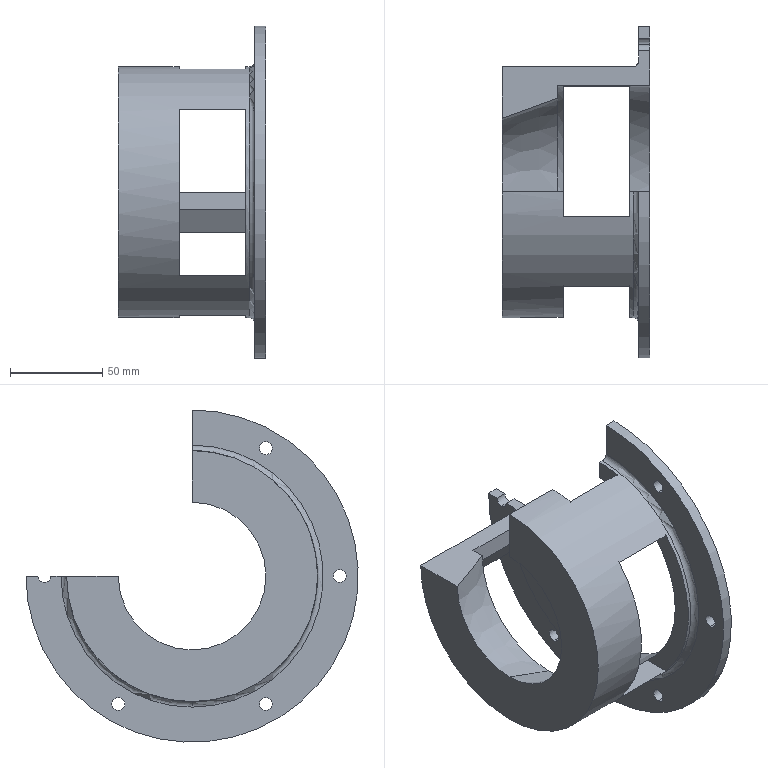Part | SolidWorks | features ICE 3, CirPattern 1, Fillet 1, Revolution 1 | 1 solid | 36 faces | box 80 x 180 x 180 mm | volume 298763 mm3 | plane 19 | cylinder 13 | torus 2 | cone 2 | commonest cylinder face diameters 7 x10 116 x1 136 x1 180 x1
STEP:
#1=CARTESIAN_POINT('',(74.,0.,-71.));
#2=VERTEX_POINT('',#1);
#3=CARTESIAN_POINT('',(74.,71.,0.));
#4=VERTEX_POINT('',#3);
#5=CARTESIAN_POINT('',(74.,0.,0.));
#6=DIRECTION('',(1.,0.,0.));
#7=DIRECTION('',(0.,0.,-1.));
#8=AXIS2_PLACEMENT_3D('',#5,#6,#7);
#9=CIRCLE('',#8,71.);
#10=EDGE_CURVE('',#2,#4,#9,.T.);
#11=ORIENTED_EDGE('',*,*,#10,.F.);
#12=CARTESIAN_POINT('',(71.,0.,-68.));
#13=VERTEX_POINT('',#12);
#14=CARTESIAN_POINT('',(71.,0.,-71.));
#15=DIRECTION('',(0.,-1.,0.));
#16=DIRECTION('',(0.,0.,-1.));
#17=AXIS2_PLACEMENT_3D('',#14,#15,#16);
#18=CIRCLE('',#17,3.);
#19=EDGE_CURVE('',#2,#13,#18,.T.);
#20=ORIENTED_EDGE('',*,*,#19,.T.);
#21=CARTESIAN_POINT('',(71.,68.,0.));
#22=VERTEX_POINT('',#21);
#23=CARTESIAN_POINT('',(71.,0.,0.));
#24=DIRECTION('',(-1.,0.,0.));
#25=DIRECTION('',(0.,0.,-1.));
#26=AXIS2_PLACEMENT_3D('',#23,#24,#25);
#27=CIRCLE('',#26,68.);
#28=EDGE_CURVE('',#22,#13,#27,.T.);
#29=ORIENTED_EDGE('',*,*,#28,.F.);
#30=CARTESIAN_POINT('',(71.,71.,0.));
#31=DIRECTION('',(0.,0.,1.));
#32=DIRECTION('',(-1.,0.,0.));
#33=AXIS2_PLACEMENT_3D('',#30,#31,#32);
#34=CIRCLE('',#33,3.);
#35=EDGE_CURVE('',#22,#4,#34,.T.);
#36=ORIENTED_EDGE('',*,*,#35,.T.);
#37=EDGE_LOOP('',(#11,#20,#29,#36));
#38=FACE_OUTER_BOUND('',#37,.T.);
#39=CARTESIAN_POINT('',(71.,0.,0.));
#40=DIRECTION('',(1.,0.,0.));
#41=DIRECTION('',(0.,0.,-1.));
#42=AXIS2_PLACEMENT_3D('',#39,#40,#41);
#43=TOROIDAL_SURFACE('',#42,71.,3.);
#44=ADVANCED_FACE('',(#38),#43,.F.);
#45=CARTESIAN_POINT('',(74.,40.,-65.782));
#46=VERTEX_POINT('',#45);
#47=CARTESIAN_POINT('',(74.,40.,-72.782));
#48=VERTEX_POINT('',#47);
#49=CARTESIAN_POINT('',(74.,40.,-69.282));
#50=DIRECTION('',(1.,0.,0.));
#51=DIRECTION('',(0.,0.,-1.));
#52=AXIS2_PLACEMENT_3D('',#49,#50,#51);
#53=CIRCLE('',#52,3.5);
#54=EDGE_CURVE('',#46,#48,#53,.T.);
#55=ORIENTED_EDGE('',*,*,#54,.F.);
#56=CARTESIAN_POINT('',(80.,40.,-65.782));
#57=VERTEX_POINT('',#56);
#58=CARTESIAN_POINT('',(70.,40.,-65.782));
#59=DIRECTION('',(1.,0.,0.));
#60=VECTOR('',#59,1000.);
#61=LINE('',#58,#60);
#62=EDGE_CURVE('',#46,#57,#61,.T.);
#63=ORIENTED_EDGE('',*,*,#62,.T.);
#64=CARTESIAN_POINT('',(80.,40.,-72.782));
#65=VERTEX_POINT('',#64);
#66=CARTESIAN_POINT('',(80.,40.,-69.282));
#67=DIRECTION('',(1.,0.,0.));
#68=DIRECTION('',(0.,0.,-1.));
#69=AXIS2_PLACEMENT_3D('',#66,#67,#68);
#70=CIRCLE('',#69,3.5);
#71=EDGE_CURVE('',#57,#65,#70,.T.);
#72=ORIENTED_EDGE('',*,*,#71,.T.);
#73=CARTESIAN_POINT('',(70.,40.,-72.782));
#74=DIRECTION('',(1.,0.,0.));
#75=VECTOR('',#74,1000.);
#76=LINE('',#73,#75);
#77=EDGE_CURVE('',#48,#65,#76,.T.);
#78=ORIENTED_EDGE('',*,*,#77,.F.);
#79=EDGE_LOOP('',(#55,#63,#72,#78));
#80=FACE_OUTER_BOUND('',#79,.T.);
#81=CARTESIAN_POINT('',(70.,40.,-69.282));
#82=DIRECTION('',(1.,0.,0.));
#83=DIRECTION('',(0.,0.,-1.));
#84=AXIS2_PLACEMENT_3D('',#81,#82,#83);
#85=CYLINDRICAL_SURFACE('',#84,3.5);
#86=ADVANCED_FACE('',(#80),#85,.F.);
#87=CARTESIAN_POINT('',(74.,-40.,-65.782));
#88=VERTEX_POINT('',#87);
#89=CARTESIAN_POINT('',(74.,-40.,-72.782));
#90=VERTEX_POINT('',#89);
#91=CARTESIAN_POINT('',(74.,-40.,-69.282));
#92=DIRECTION('',(1.,0.,0.));
#93=DIRECTION('',(0.,0.,-1.));
#94=AXIS2_PLACEMENT_3D('',#91,#92,#93);
#95=CIRCLE('',#94,3.5);
#96=EDGE_CURVE('',#88,#90,#95,.T.);
#97=ORIENTED_EDGE('',*,*,#96,.F.);
#98=CARTESIAN_POINT('',(80.,-40.,-65.782));
#99=VERTEX_POINT('',#98);
#100=CARTESIAN_POINT('',(70.,-40.,-65.782));
#101=DIRECTION('',(1.,0.,0.));
#102=VECTOR('',#101,1000.);
#103=LINE('',#100,#102);
#104=EDGE_CURVE('',#88,#99,#103,.T.);
#105=ORIENTED_EDGE('',*,*,#104,.T.);
#106=CARTESIAN_POINT('',(80.,-40.,-72.782));
#107=VERTEX_POINT('',#106);
#108=CARTESIAN_POINT('',(80.,-40.,-69.282));
#109=DIRECTION('',(1.,0.,0.));
#110=DIRECTION('',(0.,0.,-1.));
#111=AXIS2_PLACEMENT_3D('',#108,#109,#110);
#112=CIRCLE('',#111,3.5);
#113=EDGE_CURVE('',#99,#107,#112,.T.);
#114=ORIENTED_EDGE('',*,*,#113,.T.);
#115=CARTESIAN_POINT('',(70.,-40.,-72.782));
#116=DIRECTION('',(1.,0.,0.));
#117=VECTOR('',#116,1000.);
#118=LINE('',#115,#117);
#119=EDGE_CURVE('',#90,#107,#118,.T.);
#120=ORIENTED_EDGE('',*,*,#119,.F.);
#121=EDGE_LOOP('',(#97,#105,#114,#120));
#122=FACE_OUTER_BOUND('',#121,.T.);
#123=CARTESIAN_POINT('',(70.,-40.,-69.282));
#124=DIRECTION('',(1.,0.,0.));
#125=DIRECTION('',(0.,0.,-1.));
#126=AXIS2_PLACEMENT_3D('',#123,#124,#125);
#127=CYLINDRICAL_SURFACE('',#126,3.5);
#128=ADVANCED_FACE('',(#122),#127,.F.);
#129=CARTESIAN_POINT('',(74.,-80.,3.5));
#130=VERTEX_POINT('',#129);
#131=CARTESIAN_POINT('',(74.,-80.,-3.5));
#132=VERTEX_POINT('',#131);
#133=CARTESIAN_POINT('',(74.,-80.,0.));
#134=DIRECTION('',(1.,0.,0.));
#135=DIRECTION('',(0.,0.,-1.));
#136=AXIS2_PLACEMENT_3D('',#133,#134,#135);
#137=CIRCLE('',#136,3.5);
#138=EDGE_CURVE('',#130,#132,#137,.T.);
#139=ORIENTED_EDGE('',*,*,#138,.F.);
#140=CARTESIAN_POINT('',(80.,-80.,3.5));
#141=VERTEX_POINT('',#140);
#142=CARTESIAN_POINT('',(70.,-80.,3.5));
#143=DIRECTION('',(1.,0.,0.));
#144=VECTOR('',#143,1000.);
#145=LINE('',#142,#144);
#146=EDGE_CURVE('',#130,#141,#145,.T.);
#147=ORIENTED_EDGE('',*,*,#146,.T.);
#148=CARTESIAN_POINT('',(80.,-80.,-3.5));
#149=VERTEX_POINT('',#148);
#150=CARTESIAN_POINT('',(80.,-80.,0.));
#151=DIRECTION('',(1.,0.,0.));
#152=DIRECTION('',(0.,0.,-1.));
#153=AXIS2_PLACEMENT_3D('',#150,#151,#152);
#154=CIRCLE('',#153,3.5);
#155=EDGE_CURVE('',#141,#149,#154,.T.);
#156=ORIENTED_EDGE('',*,*,#155,.T.);
#157=CARTESIAN_POINT('',(70.,-80.,-3.5));
#158=DIRECTION('',(1.,0.,0.));
#159=VECTOR('',#158,1000.);
#160=LINE('',#157,#159);
#161=EDGE_CURVE('',#132,#149,#160,.T.);
#162=ORIENTED_EDGE('',*,*,#161,.F.);
#163=EDGE_LOOP('',(#139,#147,#156,#162));
#164=FACE_OUTER_BOUND('',#163,.T.);
#165=CARTESIAN_POINT('',(70.,-80.,0.));
#166=DIRECTION('',(1.,0.,0.));
#167=DIRECTION('',(0.,0.,-1.));
#168=AXIS2_PLACEMENT_3D('',#165,#166,#167);
#169=CYLINDRICAL_SURFACE('',#168,3.5);
#170=ADVANCED_FACE('',(#164),#169,.F.);
#171=CARTESIAN_POINT('',(74.,-40.,72.782));
#172=VERTEX_POINT('',#171);
#173=CARTESIAN_POINT('',(74.,-40.,65.782));
#174=VERTEX_POINT('',#173);
#175=CARTESIAN_POINT('',(74.,-40.,69.282));
#176=DIRECTION('',(1.,0.,0.));
#177=DIRECTION('',(0.,0.,-1.));
#178=AXIS2_PLACEMENT_3D('',#175,#176,#177);
#179=CIRCLE('',#178,3.5);
#180=EDGE_CURVE('',#172,#174,#179,.T.);
#181=ORIENTED_EDGE('',*,*,#180,.F.);
#182=CARTESIAN_POINT('',(80.,-40.,72.782));
#183=VERTEX_POINT('',#182);
#184=CARTESIAN_POINT('',(70.,-40.,72.782));
#185=DIRECTION('',(1.,0.,0.));
#186=VECTOR('',#185,1000.);
#187=LINE('',#184,#186);
#188=EDGE_CURVE('',#172,#183,#187,.T.);
#189=ORIENTED_EDGE('',*,*,#188,.T.);
#190=CARTESIAN_POINT('',(80.,-40.,65.782));
#191=VERTEX_POINT('',#190);
#192=CARTESIAN_POINT('',(80.,-40.,69.282));
#193=DIRECTION('',(1.,0.,0.));
#194=DIRECTION('',(0.,0.,-1.));
#195=AXIS2_PLACEMENT_3D('',#192,#193,#194);
#196=CIRCLE('',#195,3.5);
#197=EDGE_CURVE('',#183,#191,#196,.T.);
#198=ORIENTED_EDGE('',*,*,#197,.T.);
#199=CARTESIAN_POINT('',(70.,-40.,65.782));
#200=DIRECTION('',(1.,0.,0.));
#201=VECTOR('',#200,1000.);
#202=LINE('',#199,#201);
#203=EDGE_CURVE('',#174,#191,#202,.T.);
#204=ORIENTED_EDGE('',*,*,#203,.F.);
#205=EDGE_LOOP('',(#181,#189,#198,#204));
#206=FACE_OUTER_BOUND('',#205,.T.);
#207=CARTESIAN_POINT('',(70.,-40.,69.282));
#208=DIRECTION('',(1.,0.,0.));
#209=DIRECTION('',(0.,0.,-1.));
#210=AXIS2_PLACEMENT_3D('',#207,#208,#209);
#211=CYLINDRICAL_SURFACE('',#210,3.5);
#212=ADVANCED_FACE('',(#206),#211,.F.);
#213=CARTESIAN_POINT('',(74.,80.,-3.5));
#214=VERTEX_POINT('',#213);
#215=CARTESIAN_POINT('',(74.,83.5,0.));
#216=VERTEX_POINT('',#215);
#217=CARTESIAN_POINT('',(74.,80.,0.));
#218=DIRECTION('',(1.,0.,0.));
#219=DIRECTION('',(0.,0.,-1.));
#220=AXIS2_PLACEMENT_3D('',#217,#218,#219);
#221=CIRCLE('',#220,3.5);
#222=EDGE_CURVE('',#214,#216,#221,.T.);
#223=ORIENTED_EDGE('',*,*,#222,.F.);
#224=CARTESIAN_POINT('',(80.,80.,-3.5));
#225=VERTEX_POINT('',#224);
#226=CARTESIAN_POINT('',(70.,80.,-3.5));
#227=DIRECTION('',(1.,0.,0.));
#228=VECTOR('',#227,1000.);
#229=LINE('',#226,#228);
#230=EDGE_CURVE('',#214,#225,#229,.T.);
#231=ORIENTED_EDGE('',*,*,#230,.T.);
#232=CARTESIAN_POINT('',(80.,83.5,0.));
#233=VERTEX_POINT('',#232);
#234=CARTESIAN_POINT('',(80.,80.,0.));
#235=DIRECTION('',(1.,0.,0.));
#236=DIRECTION('',(0.,0.,-1.));
#237=AXIS2_PLACEMENT_3D('',#234,#235,#236);
#238=CIRCLE('',#237,3.5);
#239=EDGE_CURVE('',#225,#233,#238,.T.);
#240=ORIENTED_EDGE('',*,*,#239,.T.);
#241=CARTESIAN_POINT('',(70.,83.5,0.));
#242=DIRECTION('',(-1.,0.,0.));
#243=VECTOR('',#242,1000.);
#244=LINE('',#241,#243);
#245=EDGE_CURVE('',#233,#216,#244,.T.);
#246=ORIENTED_EDGE('',*,*,#245,.T.);
#247=EDGE_LOOP('',(#223,#231,#240,#246));
#248=FACE_OUTER_BOUND('',#247,.T.);
#249=CARTESIAN_POINT('',(70.,80.,0.));
#250=DIRECTION('',(1.,0.,0.));
#251=DIRECTION('',(0.,0.,-1.));
#252=AXIS2_PLACEMENT_3D('',#249,#250,#251);
#253=CYLINDRICAL_SURFACE('',#252,3.5);
#254=ADVANCED_FACE('',(#248),#253,.F.);
#255=CARTESIAN_POINT('',(0.,40.,0.));
#256=VERTEX_POINT('',#255);
#257=CARTESIAN_POINT('',(0.,0.,-40.));
#258=VERTEX_POINT('',#257);
#259=CARTESIAN_POINT('',(0.,0.,0.));
#260=DIRECTION('',(-1.,0.,0.));
#261=DIRECTION('',(0.,0.,1.));
#262=AXIS2_PLACEMENT_3D('',#259,#260,#261);
#263=CIRCLE('',#262,40.);
#264=EDGE_CURVE('',#256,#258,#263,.T.);
#265=ORIENTED_EDGE('',*,*,#264,.T.);
#266=CARTESIAN_POINT('',(30.,0.,-50.919));
#267=VERTEX_POINT('',#266);
#268=CARTESIAN_POINT('',(0.,0.,-40.));
#269=DIRECTION('',(0.9397,0.,-0.342));
#270=VECTOR('',#269,1000.);
#271=LINE('',#268,#270);
#272=EDGE_CURVE('',#258,#267,#271,.T.);
#273=ORIENTED_EDGE('',*,*,#272,.T.);
#274=CARTESIAN_POINT('',(30.,50.919,0.));
#275=VERTEX_POINT('',#274);
#276=CARTESIAN_POINT('',(30.,0.,0.));
#277=DIRECTION('',(-1.,0.,0.));
#278=DIRECTION('',(0.,0.,1.));
#279=AXIS2_PLACEMENT_3D('',#276,#277,#278);
#280=CIRCLE('',#279,50.919);
#281=EDGE_CURVE('',#275,#267,#280,.T.);
#282=ORIENTED_EDGE('',*,*,#281,.F.);
#283=CARTESIAN_POINT('',(-109.899,0.,0.));
#284=DIRECTION('',(-0.9397,-0.342,0.));
#285=VECTOR('',#284,1000.);
#286=LINE('',#283,#285);
#287=EDGE_CURVE('',#275,#256,#286,.T.);
#288=ORIENTED_EDGE('',*,*,#287,.T.);
#289=EDGE_LOOP('',(#265,#273,#282,#288));
#290=FACE_OUTER_BOUND('',#289,.T.);
#291=CARTESIAN_POINT('',(0.,0.,0.));
#292=DIRECTION('',(1.,0.,0.));
#293=DIRECTION('',(0.,0.,-1.));
#294=AXIS2_PLACEMENT_3D('',#291,#292,#293);
#295=CONICAL_SURFACE('',#294,40.,0.3491);
#296=ADVANCED_FACE('',(#290),#295,.F.);
#297=ORIENTED_EDGE('',*,*,#272,.F.);
#298=CARTESIAN_POINT('',(0.,0.,40.));
#299=VERTEX_POINT('',#298);
#300=CARTESIAN_POINT('',(0.,0.,0.));
#301=DIRECTION('',(-1.,0.,0.));
#302=DIRECTION('',(0.,0.,1.));
#303=AXIS2_PLACEMENT_3D('',#300,#301,#302);
#304=CIRCLE('',#303,40.);
#305=EDGE_CURVE('',#258,#299,#304,.T.);
#306=ORIENTED_EDGE('',*,*,#305,.T.);
#307=CARTESIAN_POINT('',(30.,0.,50.919));
#308=VERTEX_POINT('',#307);
#309=CARTESIAN_POINT('',(-109.899,0.,0.));
#310=DIRECTION('',(0.9397,0.,0.342));
#311=VECTOR('',#310,1000.);
#312=LINE('',#309,#311);
#313=EDGE_CURVE('',#299,#308,#312,.T.);
#314=ORIENTED_EDGE('',*,*,#313,.T.);
#315=CARTESIAN_POINT('',(30.,0.,0.));
#316=DIRECTION('',(-1.,0.,0.));
#317=DIRECTION('',(0.,0.,1.));
#318=AXIS2_PLACEMENT_3D('',#315,#316,#317);
#319=CIRCLE('',#318,50.919);
#320=EDGE_CURVE('',#267,#308,#319,.T.);
#321=ORIENTED_EDGE('',*,*,#320,.F.);
#322=EDGE_LOOP('',(#297,#306,#314,#321));
#323=FACE_OUTER_BOUND('',#322,.T.);
#324=CARTESIAN_POINT('',(0.,0.,0.));
#325=DIRECTION('',(1.,0.,0.));
#326=DIRECTION('',(0.,0.,-1.));
#327=AXIS2_PLACEMENT_3D('',#324,#325,#326);
#328=CONICAL_SURFACE('',#327,40.,0.3491);
#329=ADVANCED_FACE('',(#323),#328,.F.);
#330=ORIENTED_EDGE('',*,*,#264,.F.);
#331=CARTESIAN_POINT('',(0.,68.,0.));
#332=VERTEX_POINT('',#331);
#333=CARTESIAN_POINT('',(0.,0.,0.));
#334=DIRECTION('',(0.,-1.,0.));
#335=VECTOR('',#334,1000.);
#336=LINE('',#333,#335);
#337=EDGE_CURVE('',#332,#256,#336,.T.);
#338=ORIENTED_EDGE('',*,*,#337,.F.);
#339=CARTESIAN_POINT('',(0.,0.,68.));
#340=VERTEX_POINT('',#339);
#341=CARTESIAN_POINT('',(0.,0.,0.));
#342=DIRECTION('',(-1.,0.,0.));
#343=DIRECTION('',(0.,0.,1.));
#344=AXIS2_PLACEMENT_3D('',#341,#342,#343);
#345=CIRCLE('',#344,68.);
#346=EDGE_CURVE('',#332,#340,#345,.T.);
#347=ORIENTED_EDGE('',*,*,#346,.T.);
#348=CARTESIAN_POINT('',(0.,0.,0.));
#349=DIRECTION('',(0.,0.,1.));
#350=VECTOR('',#349,1000.);
#351=LINE('',#348,#350);
#352=EDGE_CURVE('',#299,#340,#351,.T.);
#353=ORIENTED_EDGE('',*,*,#352,.F.);
#354=ORIENTED_EDGE('',*,*,#305,.F.);
#355=EDGE_LOOP('',(#330,#338,#347,#353,#354));
#356=FACE_OUTER_BOUND('',#355,.T.);
#357=CARTESIAN_POINT('',(0.,40.,0.));
#358=DIRECTION('',(1.,0.,0.));
#359=DIRECTION('',(0.,0.,-1.));
#360=AXIS2_PLACEMENT_3D('',#357,#358,#359);
#361=PLANE('',#360);
#362=ADVANCED_FACE('',(#356),#361,.F.);
#363=CARTESIAN_POINT('',(33.,64.461,-21.65));
#364=VERTEX_POINT('',#363);
#365=CARTESIAN_POINT('',(33.,-13.481,-66.65));
#366=VERTEX_POINT('',#365);
#367=CARTESIAN_POINT('',(33.,0.,0.));
#368=DIRECTION('',(-1.,0.,0.));
#369=DIRECTION('',(0.,-1.,0.));
#370=AXIS2_PLACEMENT_3D('',#367,#368,#369);
#371=CIRCLE('',#370,68.);
#372=EDGE_CURVE('',#364,#366,#371,.T.);
#373=ORIENTED_EDGE('',*,*,#372,.T.);
#374=CARTESIAN_POINT('',(69.,-13.481,-66.65));
#375=VERTEX_POINT('',#374);
#376=CARTESIAN_POINT('',(0.,-13.481,-66.65));
#377=DIRECTION('',(1.,0.,0.));
#378=VECTOR('',#377,1000.);
#379=LINE('',#376,#378);
#380=EDGE_CURVE('',#366,#375,#379,.T.);
#381=ORIENTED_EDGE('',*,*,#380,.T.);
#382=CARTESIAN_POINT('',(69.,64.461,-21.65));
#383=VERTEX_POINT('',#382);
#384=CARTESIAN_POINT('',(69.,0.,0.));
#385=DIRECTION('',(1.,0.,0.));
#386=DIRECTION('',(0.,1.,0.));
#387=AXIS2_PLACEMENT_3D('',#384,#385,#386);
#388=CIRCLE('',#387,68.);
#389=EDGE_CURVE('',#375,#383,#388,.T.);
#390=ORIENTED_EDGE('',*,*,#389,.T.);
#391=CARTESIAN_POINT('',(0.,64.461,-21.65));
#392=DIRECTION('',(-1.,0.,0.));
#393=VECTOR('',#392,1000.);
#394=LINE('',#391,#393);
#395=EDGE_CURVE('',#383,#364,#394,.T.);
#396=ORIENTED_EDGE('',*,*,#395,.T.);
#397=EDGE_LOOP('',(#373,#381,#390,#396));
#398=FACE_BOUND('',#397,.T.);
#399=CARTESIAN_POINT('',(33.,-50.98,45.));
#400=VERTEX_POINT('',#399);
#401=CARTESIAN_POINT('',(69.,-50.98,45.));
#402=VERTEX_POINT('',#401);
#403=CARTESIAN_POINT('',(0.,-50.98,45.));
#404=DIRECTION('',(1.,0.,0.));
#405=VECTOR('',#404,1000.);
#406=LINE('',#403,#405);
#407=EDGE_CURVE('',#400,#402,#406,.T.);
#408=ORIENTED_EDGE('',*,*,#407,.T.);
#409=CARTESIAN_POINT('',(69.,-50.98,-45.));
#410=VERTEX_POINT('',#409);
#411=CARTESIAN_POINT('',(69.,0.,0.));
#412=DIRECTION('',(1.,0.,0.));
#413=DIRECTION('',(0.,0.,-1.));
#414=AXIS2_PLACEMENT_3D('',#411,#412,#413);
#415=CIRCLE('',#414,68.);
#416=EDGE_CURVE('',#402,#410,#415,.T.);
#417=ORIENTED_EDGE('',*,*,#416,.T.);
#418=CARTESIAN_POINT('',(33.,-50.98,-45.));
#419=VERTEX_POINT('',#418);
#420=CARTESIAN_POINT('',(0.,-50.98,-45.));
#421=DIRECTION('',(-1.,0.,0.));
#422=VECTOR('',#421,1000.);
#423=LINE('',#420,#422);
#424=EDGE_CURVE('',#410,#419,#423,.T.);
#425=ORIENTED_EDGE('',*,*,#424,.T.);
#426=CARTESIAN_POINT('',(33.,0.,0.));
#427=DIRECTION('',(-1.,0.,0.));
#428=DIRECTION('',(0.,0.,1.));
#429=AXIS2_PLACEMENT_3D('',#426,#427,#428);
#430=CIRCLE('',#429,68.);
#431=EDGE_CURVE('',#419,#400,#430,.T.);
#432=ORIENTED_EDGE('',*,*,#431,.T.);
#433=EDGE_LOOP('',(#408,#417,#425,#432));
#434=FACE_BOUND('',#433,.T.);
#435=ORIENTED_EDGE('',*,*,#346,.F.);
#436=CARTESIAN_POINT('',(0.,68.,0.));
#437=DIRECTION('',(1.,0.,0.));
#438=VECTOR('',#437,1000.);
#439=LINE('',#436,#438);
#440=EDGE_CURVE('',#332,#22,#439,.T.);
#441=ORIENTED_EDGE('',*,*,#440,.T.);
#442=ORIENTED_EDGE('',*,*,#28,.T.);
#443=CARTESIAN_POINT('',(71.,0.,68.));
#444=VERTEX_POINT('',#443);
#445=CARTESIAN_POINT('',(71.,0.,0.));
#446=DIRECTION('',(-1.,0.,0.));
#447=DIRECTION('',(0.,0.,-1.));
#448=AXIS2_PLACEMENT_3D('',#445,#446,#447);
#449=CIRCLE('',#448,68.);
#450=EDGE_CURVE('',#13,#444,#449,.T.);
#451=ORIENTED_EDGE('',*,*,#450,.T.);
#452=CARTESIAN_POINT('',(69.,0.,68.));
#453=VERTEX_POINT('',#452);
#454=CARTESIAN_POINT('',(0.,0.,68.));
#455=DIRECTION('',(-1.,0.,0.));
#456=VECTOR('',#455,1000.);
#457=LINE('',#454,#456);
#458=EDGE_CURVE('',#444,#453,#457,.T.);
#459=ORIENTED_EDGE('',*,*,#458,.T.);
#460=CARTESIAN_POINT('',(69.,-13.481,66.65));
#461=VERTEX_POINT('',#460);
#462=CARTESIAN_POINT('',(69.,0.,0.));
#463=DIRECTION('',(1.,0.,0.));
#464=DIRECTION('',(0.,1.,0.));
#465=AXIS2_PLACEMENT_3D('',#462,#463,#464);
#466=CIRCLE('',#465,68.);
#467=EDGE_CURVE('',#453,#461,#466,.T.);
#468=ORIENTED_EDGE('',*,*,#467,.T.);
#469=CARTESIAN_POINT('',(33.,-13.481,66.65));
#470=VERTEX_POINT('',#469);
#471=CARTESIAN_POINT('',(0.,-13.481,66.65));
#472=DIRECTION('',(-1.,0.,0.));
#473=VECTOR('',#472,1000.);
#474=LINE('',#471,#473);
#475=EDGE_CURVE('',#461,#470,#474,.T.);
#476=ORIENTED_EDGE('',*,*,#475,.T.);
#477=CARTESIAN_POINT('',(33.,0.,68.));
#478=VERTEX_POINT('',#477);
#479=CARTESIAN_POINT('',(33.,0.,0.));
#480=DIRECTION('',(-1.,0.,0.));
#481=DIRECTION('',(0.,-1.,0.));
#482=AXIS2_PLACEMENT_3D('',#479,#480,#481);
#483=CIRCLE('',#482,68.);
#484=EDGE_CURVE('',#470,#478,#483,.T.);
#485=ORIENTED_EDGE('',*,*,#484,.T.);
#486=CARTESIAN_POINT('',(0.,0.,68.));
#487=DIRECTION('',(-1.,0.,0.));
#488=VECTOR('',#487,1000.);
#489=LINE('',#486,#488);
#490=EDGE_CURVE('',#478,#340,#489,.T.);
#491=ORIENTED_EDGE('',*,*,#490,.T.);
#492=EDGE_LOOP('',(#435,#441,#442,#451,#459,#468,#476,#485,#491));
#493=FACE_OUTER_BOUND('',#492,.T.);
#494=CARTESIAN_POINT('',(0.,0.,0.));
#495=DIRECTION('',(-1.,0.,0.));
#496=DIRECTION('',(0.,0.,1.));
#497=AXIS2_PLACEMENT_3D('',#494,#495,#496);
#498=CYLINDRICAL_SURFACE('',#497,68.);
#499=ADVANCED_FACE('',(#398,#434,#493),#498,.T.);
#500=CARTESIAN_POINT('',(74.,40.,-69.282));
#501=DIRECTION('',(1.,0.,0.));
#502=DIRECTION('',(0.,0.,-1.));
#503=AXIS2_PLACEMENT_3D('',#500,#501,#502);
#504=CIRCLE('',#503,3.5);
#505=EDGE_CURVE('',#48,#46,#504,.T.);
#506=ORIENTED_EDGE('',*,*,#505,.T.);
#507=ORIENTED_EDGE('',*,*,#54,.T.);
#508=EDGE_LOOP('',(#506,#507));
#509=FACE_BOUND('',#508,.T.);
#510=CARTESIAN_POINT('',(74.,-40.,-69.282));
#511=DIRECTION('',(1.,0.,0.));
#512=DIRECTION('',(0.,0.,-1.));
#513=AXIS2_PLACEMENT_3D('',#510,#511,#512);
#514=CIRCLE('',#513,3.5);
#515=EDGE_CURVE('',#90,#88,#514,.T.);
#516=ORIENTED_EDGE('',*,*,#515,.T.);
#517=ORIENTED_EDGE('',*,*,#96,.T.);
#518=EDGE_LOOP('',(#516,#517));
#519=FACE_BOUND('',#518,.T.);
#520=CARTESIAN_POINT('',(74.,-80.,0.));
#521=DIRECTION('',(1.,0.,0.));
#522=DIRECTION('',(0.,0.,-1.));
#523=AXIS2_PLACEMENT_3D('',#520,#521,#522);
#524=CIRCLE('',#523,3.5);
#525=EDGE_CURVE('',#132,#130,#524,.T.);
#526=ORIENTED_EDGE('',*,*,#525,.T.);
#527=ORIENTED_EDGE('',*,*,#138,.T.);
#528=EDGE_LOOP('',(#526,#527));
#529=FACE_BOUND('',#528,.T.);
#530=CARTESIAN_POINT('',(74.,-40.,69.282));
#531=DIRECTION('',(1.,0.,0.));
#532=DIRECTION('',(0.,0.,-1.));
#533=AXIS2_PLACEMENT_3D('',#530,#531,#532);
#534=CIRCLE('',#533,3.5);
#535=EDGE_CURVE('',#174,#172,#534,.T.);
#536=ORIENTED_EDGE('',*,*,#535,.T.);
#537=ORIENTED_EDGE('',*,*,#180,.T.);
#538=EDGE_LOOP('',(#536,#537));
#539=FACE_BOUND('',#538,.T.);
#540=CARTESIAN_POINT('',(74.,0.,71.));
#541=VERTEX_POINT('',#540);
#542=CARTESIAN_POINT('',(74.,0.,0.));
#543=DIRECTION('',(1.,0.,0.));
#544=DIRECTION('',(0.,0.,-1.));
#545=AXIS2_PLACEMENT_3D('',#542,#543,#544);
#546=CIRCLE('',#545,71.);
#547=EDGE_CURVE('',#541,#2,#546,.T.);
#548=ORIENTED_EDGE('',*,*,#547,.T.);
#549=ORIENTED_EDGE('',*,*,#10,.T.);
#550=CARTESIAN_POINT('',(74.,76.5,0.));
#551=VERTEX_POINT('',#550);
#552=CARTESIAN_POINT('',(74.,68.,0.));
#553=DIRECTION('',(0.,1.,0.));
#554=VECTOR('',#553,1000.);
#555=LINE('',#552,#554);
#556=EDGE_CURVE('',#4,#551,#555,.T.);
#557=ORIENTED_EDGE('',*,*,#556,.T.);
#558=CARTESIAN_POINT('',(74.,80.,0.));
#559=DIRECTION('',(1.,0.,0.));
#560=DIRECTION('',(0.,0.,-1.));
#561=AXIS2_PLACEMENT_3D('',#558,#559,#560);
#562=CIRCLE('',#561,3.5);
#563=EDGE_CURVE('',#551,#214,#562,.T.);
#564=ORIENTED_EDGE('',*,*,#563,.T.);
#565=ORIENTED_EDGE('',*,*,#222,.T.);
#566=CARTESIAN_POINT('',(74.,90.,0.));
#567=VERTEX_POINT('',#566);
#568=CARTESIAN_POINT('',(74.,68.,0.));
#569=DIRECTION('',(0.,1.,0.));
#570=VECTOR('',#569,1000.);
#571=LINE('',#568,#570);
#572=EDGE_CURVE('',#216,#567,#571,.T.);
#573=ORIENTED_EDGE('',*,*,#572,.T.);
#574=CARTESIAN_POINT('',(74.,0.,90.));
#575=VERTEX_POINT('',#574);
#576=CARTESIAN_POINT('',(74.,0.,0.));
#577=DIRECTION('',(-1.,0.,0.));
#578=DIRECTION('',(0.,0.,1.));
#579=AXIS2_PLACEMENT_3D('',#576,#577,#578);
#580=CIRCLE('',#579,90.);
#581=EDGE_CURVE('',#567,#575,#580,.T.);
#582=ORIENTED_EDGE('',*,*,#581,.T.);
#583=CARTESIAN_POINT('',(74.,0.,0.));
#584=DIRECTION('',(0.,0.,-1.));
#585=VECTOR('',#584,1000.);
#586=LINE('',#583,#585);
#587=EDGE_CURVE('',#575,#541,#586,.T.);
#588=ORIENTED_EDGE('',*,*,#587,.T.);
#589=EDGE_LOOP('',(#548,#549,#557,#564,#565,#573,#582,#588));
#590=FACE_OUTER_BOUND('',#589,.T.);
#591=CARTESIAN_POINT('',(74.,68.,0.));
#592=DIRECTION('',(1.,0.,0.));
#593=DIRECTION('',(0.,0.,-1.));
#594=AXIS2_PLACEMENT_3D('',#591,#592,#593);
#595=PLANE('',#594);
#596=ADVANCED_FACE('',(#509,#519,#529,#539,#590),#595,.F.);
#597=ORIENTED_EDGE('',*,*,#581,.F.);
#598=CARTESIAN_POINT('',(80.,90.,0.));
#599=VERTEX_POINT('',#598);
#600=CARTESIAN_POINT('',(0.,90.,0.));
#601=DIRECTION('',(1.,0.,0.));
#602=VECTOR('',#601,1000.);
#603=LINE('',#600,#602);
#604=EDGE_CURVE('',#567,#599,#603,.T.);
#605=ORIENTED_EDGE('',*,*,#604,.T.);
#606=CARTESIAN_POINT('',(80.,0.,90.));
#607=VERTEX_POINT('',#606);
#608=CARTESIAN_POINT('',(80.,0.,0.));
#609=DIRECTION('',(-1.,0.,0.));
#610=DIRECTION('',(0.,0.,1.));
#611=AXIS2_PLACEMENT_3D('',#608,#609,#610);
#612=CIRCLE('',#611,90.);
#613=EDGE_CURVE('',#599,#607,#612,.T.);
#614=ORIENTED_EDGE('',*,*,#613,.T.);
#615=CARTESIAN_POINT('',(0.,0.,90.));
#616=DIRECTION('',(-1.,0.,0.));
#617=VECTOR('',#616,1000.);
#618=LINE('',#615,#617);
#619=EDGE_CURVE('',#607,#575,#618,.T.);
#620=ORIENTED_EDGE('',*,*,#619,.T.);
#621=EDGE_LOOP('',(#597,#605,#614,#620));
#622=FACE_OUTER_BOUND('',#621,.T.);
#623=CARTESIAN_POINT('',(0.,0.,0.));
#624=DIRECTION('',(-1.,0.,0.));
#625=DIRECTION('',(0.,0.,1.));
#626=AXIS2_PLACEMENT_3D('',#623,#624,#625);
#627=CYLINDRICAL_SURFACE('',#626,90.);
#628=ADVANCED_FACE('',(#622),#627,.T.);
#629=CARTESIAN_POINT('',(80.,40.,-69.282));
#630=DIRECTION('',(1.,0.,0.));
#631=DIRECTION('',(0.,0.,-1.));
#632=AXIS2_PLACEMENT_3D('',#629,#630,#631);
#633=CIRCLE('',#632,3.5);
#634=EDGE_CURVE('',#65,#57,#633,.T.);
#635=ORIENTED_EDGE('',*,*,#634,.F.);
#636=ORIENTED_EDGE('',*,*,#71,.F.);
#637=EDGE_LOOP('',(#635,#636));
#638=FACE_BOUND('',#637,.T.);
#639=CARTESIAN_POINT('',(80.,-40.,-69.282));
#640=DIRECTION('',(1.,0.,0.));
#641=DIRECTION('',(0.,0.,-1.));
#642=AXIS2_PLACEMENT_3D('',#639,#640,#641);
#643=CIRCLE('',#642,3.5);
#644=EDGE_CURVE('',#107,#99,#643,.T.);
#645=ORIENTED_EDGE('',*,*,#644,.F.);
#646=ORIENTED_EDGE('',*,*,#113,.F.);
#647=EDGE_LOOP('',(#645,#646));
#648=FACE_BOUND('',#647,.T.);
#649=CARTESIAN_POINT('',(80.,-80.,0.));
#650=DIRECTION('',(1.,0.,0.));
#651=DIRECTION('',(0.,0.,-1.));
#652=AXIS2_PLACEMENT_3D('',#649,#650,#651);
#653=CIRCLE('',#652,3.5);
#654=EDGE_CURVE('',#149,#141,#653,.T.);
#655=ORIENTED_EDGE('',*,*,#654,.F.);
#656=ORIENTED_EDGE('',*,*,#155,.F.);
#657=EDGE_LOOP('',(#655,#656));
#658=FACE_BOUND('',#657,.T.);
#659=CARTESIAN_POINT('',(80.,-40.,69.282));
#660=DIRECTION('',(1.,0.,0.));
#661=DIRECTION('',(0.,0.,-1.));
#662=AXIS2_PLACEMENT_3D('',#659,#660,#661);
#663=CIRCLE('',#662,3.5);
#664=EDGE_CURVE('',#191,#183,#663,.T.);
#665=ORIENTED_EDGE('',*,*,#664,.F.);
#666=ORIENTED_EDGE('',*,*,#197,.F.);
#667=EDGE_LOOP('',(#665,#666));
#668=FACE_BOUND('',#667,.T.);
#669=ORIENTED_EDGE('',*,*,#613,.F.);
#670=CARTESIAN_POINT('',(80.,0.,0.));
#671=DIRECTION('',(0.,-1.,0.));
#672=VECTOR('',#671,1000.);
#673=LINE('',#670,#672);
#674=EDGE_CURVE('',#599,#233,#673,.T.);
#675=ORIENTED_EDGE('',*,*,#674,.T.);
#676=ORIENTED_EDGE('',*,*,#239,.F.);
#677=CARTESIAN_POINT('',(80.,76.5,0.));
#678=VERTEX_POINT('',#677);
#679=CARTESIAN_POINT('',(80.,80.,0.));
#680=DIRECTION('',(1.,0.,0.));
#681=DIRECTION('',(0.,0.,-1.));
#682=AXIS2_PLACEMENT_3D('',#679,#680,#681);
#683=CIRCLE('',#682,3.5);
#684=EDGE_CURVE('',#678,#225,#683,.T.);
#685=ORIENTED_EDGE('',*,*,#684,.F.);
#686=CARTESIAN_POINT('',(80.,58.,0.));
#687=VERTEX_POINT('',#686);
#688=CARTESIAN_POINT('',(80.,0.,0.));
#689=DIRECTION('',(0.,-1.,0.));
#690=VECTOR('',#689,1000.);
#691=LINE('',#688,#690);
#692=EDGE_CURVE('',#678,#687,#691,.T.);
#693=ORIENTED_EDGE('',*,*,#692,.T.);
#694=CARTESIAN_POINT('',(80.,0.,58.));
#695=VERTEX_POINT('',#694);
#696=CARTESIAN_POINT('',(80.,0.,0.));
#697=DIRECTION('',(-1.,0.,0.));
#698=DIRECTION('',(0.,0.,1.));
#699=AXIS2_PLACEMENT_3D('',#696,#697,#698);
#700=CIRCLE('',#699,58.);
#701=EDGE_CURVE('',#687,#695,#700,.T.);
#702=ORIENTED_EDGE('',*,*,#701,.T.);
#703=CARTESIAN_POINT('',(80.,0.,0.));
#704=DIRECTION('',(0.,0.,1.));
#705=VECTOR('',#704,1000.);
#706=LINE('',#703,#705);
#707=EDGE_CURVE('',#695,#607,#706,.T.);
#708=ORIENTED_EDGE('',*,*,#707,.T.);
#709=EDGE_LOOP('',(#669,#675,#676,#685,#693,#702,#708));
#710=FACE_OUTER_BOUND('',#709,.T.);
#711=CARTESIAN_POINT('',(80.,90.,0.));
#712=DIRECTION('',(-1.,0.,0.));
#713=DIRECTION('',(0.,0.,1.));
#714=AXIS2_PLACEMENT_3D('',#711,#712,#713);
#715=PLANE('',#714);
#716=ADVANCED_FACE('',(#638,#648,#658,#668,#710),#715,.F.);
#717=CARTESIAN_POINT('',(69.,57.267,-9.19));
#718=VERTEX_POINT('',#717);
#719=CARTESIAN_POINT('',(69.,-20.675,-54.19));
#720=VERTEX_POINT('',#719);
#721=CARTESIAN_POINT('',(69.,0.,0.));
#722=DIRECTION('',(-1.,0.,0.));
#723=DIRECTION('',(0.,1.,0.));
#724=AXIS2_PLACEMENT_3D('',#721,#722,#723);
#725=CIRCLE('',#724,58.);
#726=EDGE_CURVE('',#718,#720,#725,.T.);
#727=ORIENTED_EDGE('',*,*,#726,.T.);
#728=CARTESIAN_POINT('',(33.,-20.675,-54.19));
#729=VERTEX_POINT('',#728);
#730=CARTESIAN_POINT('',(0.,-20.675,-54.19));
#731=DIRECTION('',(-1.,0.,0.));
#732=VECTOR('',#731,1000.);
#733=LINE('',#730,#732);
#734=EDGE_CURVE('',#720,#729,#733,.T.);
#735=ORIENTED_EDGE('',*,*,#734,.T.);
#736=CARTESIAN_POINT('',(33.,57.267,-9.19));
#737=VERTEX_POINT('',#736);
#738=CARTESIAN_POINT('',(33.,0.,0.));
#739=DIRECTION('',(1.,0.,0.));
#740=DIRECTION('',(0.,-1.,0.));
#741=AXIS2_PLACEMENT_3D('',#738,#739,#740);
#742=CIRCLE('',#741,58.);
#743=EDGE_CURVE('',#729,#737,#742,.T.);
#744=ORIENTED_EDGE('',*,*,#743,.T.);
#745=CARTESIAN_POINT('',(0.,57.267,-9.19));
#746=DIRECTION('',(1.,0.,0.));
#747=VECTOR('',#746,1000.);
#748=LINE('',#745,#747);
#749=EDGE_CURVE('',#737,#718,#748,.T.);
#750=ORIENTED_EDGE('',*,*,#749,.T.);
#751=EDGE_LOOP('',(#727,#735,#744,#750));
#752=FACE_BOUND('',#751,.T.);
#753=CARTESIAN_POINT('',(33.,-36.592,-45.));
#754=VERTEX_POINT('',#753);
#755=CARTESIAN_POINT('',(69.,-36.592,-45.));
#756=VERTEX_POINT('',#755);
#757=CARTESIAN_POINT('',(0.,-36.592,-45.));
#758=DIRECTION('',(1.,0.,0.));
#759=VECTOR('',#758,1000.);
#760=LINE('',#757,#759);
#761=EDGE_CURVE('',#754,#756,#760,.T.);
#762=ORIENTED_EDGE('',*,*,#761,.T.);
#763=CARTESIAN_POINT('',(69.,-36.592,45.));
#764=VERTEX_POINT('',#763);
#765=CARTESIAN_POINT('',(69.,0.,0.));
#766=DIRECTION('',(-1.,0.,0.));
#767=DIRECTION('',(0.,0.,-1.));
#768=AXIS2_PLACEMENT_3D('',#765,#766,#767);
#769=CIRCLE('',#768,58.);
#770=EDGE_CURVE('',#756,#764,#769,.T.);
#771=ORIENTED_EDGE('',*,*,#770,.T.);
#772=CARTESIAN_POINT('',(33.,-36.592,45.));
#773=VERTEX_POINT('',#772);
#774=CARTESIAN_POINT('',(0.,-36.592,45.));
#775=DIRECTION('',(-1.,0.,0.));
#776=VECTOR('',#775,1000.);
#777=LINE('',#774,#776);
#778=EDGE_CURVE('',#764,#773,#777,.T.);
#779=ORIENTED_EDGE('',*,*,#778,.T.);
#780=CARTESIAN_POINT('',(33.,0.,0.));
#781=DIRECTION('',(1.,0.,0.));
#782=DIRECTION('',(0.,0.,1.));
#783=AXIS2_PLACEMENT_3D('',#780,#781,#782);
#784=CIRCLE('',#783,58.);
#785=EDGE_CURVE('',#773,#754,#784,.T.);
#786=ORIENTED_EDGE('',*,*,#785,.T.);
#787=EDGE_LOOP('',(#762,#771,#779,#786));
#788=FACE_BOUND('',#787,.T.);
#789=ORIENTED_EDGE('',*,*,#701,.F.);
#790=CARTESIAN_POINT('',(30.,58.,0.));
#791=VERTEX_POINT('',#790);
#792=CARTESIAN_POINT('',(0.,58.,0.));
#793=DIRECTION('',(-1.,0.,0.));
#794=VECTOR('',#793,1000.);
#795=LINE('',#792,#794);
#796=EDGE_CURVE('',#687,#791,#795,.T.);
#797=ORIENTED_EDGE('',*,*,#796,.T.);
#798=CARTESIAN_POINT('',(30.,0.,58.));
#799=VERTEX_POINT('',#798);
#800=CARTESIAN_POINT('',(30.,0.,0.));
#801=DIRECTION('',(-1.,0.,0.));
#802=DIRECTION('',(0.,0.,1.));
#803=AXIS2_PLACEMENT_3D('',#800,#801,#802);
#804=CIRCLE('',#803,58.);
#805=EDGE_CURVE('',#791,#799,#804,.T.);
#806=ORIENTED_EDGE('',*,*,#805,.T.);
#807=CARTESIAN_POINT('',(33.,0.,58.));
#808=VERTEX_POINT('',#807);
#809=CARTESIAN_POINT('',(0.,0.,58.));
#810=DIRECTION('',(1.,0.,0.));
#811=VECTOR('',#810,1000.);
#812=LINE('',#809,#811);
#813=EDGE_CURVE('',#799,#808,#812,.T.);
#814=ORIENTED_EDGE('',*,*,#813,.T.);
#815=CARTESIAN_POINT('',(33.,-20.675,54.19));
#816=VERTEX_POINT('',#815);
#817=CARTESIAN_POINT('',(33.,0.,0.));
#818=DIRECTION('',(1.,0.,0.));
#819=DIRECTION('',(0.,-1.,0.));
#820=AXIS2_PLACEMENT_3D('',#817,#818,#819);
#821=CIRCLE('',#820,58.);
#822=EDGE_CURVE('',#808,#816,#821,.T.);
#823=ORIENTED_EDGE('',*,*,#822,.T.);
#824=CARTESIAN_POINT('',(69.,-20.675,54.19));
#825=VERTEX_POINT('',#824);
#826=CARTESIAN_POINT('',(0.,-20.675,54.19));
#827=DIRECTION('',(1.,0.,0.));
#828=VECTOR('',#827,1000.);
#829=LINE('',#826,#828);
#830=EDGE_CURVE('',#816,#825,#829,.T.);
#831=ORIENTED_EDGE('',*,*,#830,.T.);
#832=CARTESIAN_POINT('',(69.,0.,58.));
#833=VERTEX_POINT('',#832);
#834=CARTESIAN_POINT('',(69.,0.,0.));
#835=DIRECTION('',(-1.,0.,0.));
#836=DIRECTION('',(0.,1.,0.));
#837=AXIS2_PLACEMENT_3D('',#834,#835,#836);
#838=CIRCLE('',#837,58.);
#839=EDGE_CURVE('',#825,#833,#838,.T.);
#840=ORIENTED_EDGE('',*,*,#839,.T.);
#841=CARTESIAN_POINT('',(0.,0.,58.));
#842=DIRECTION('',(1.,0.,0.));
#843=VECTOR('',#842,1000.);
#844=LINE('',#841,#843);
#845=EDGE_CURVE('',#833,#695,#844,.T.);
#846=ORIENTED_EDGE('',*,*,#845,.T.);
#847=EDGE_LOOP('',(#789,#797,#806,#814,#823,#831,#840,#846));
#848=FACE_OUTER_BOUND('',#847,.T.);
#849=CARTESIAN_POINT('',(0.,0.,0.));
#850=DIRECTION('',(-1.,0.,0.));
#851=DIRECTION('',(0.,0.,1.));
#852=AXIS2_PLACEMENT_3D('',#849,#850,#851);
#853=CYLINDRICAL_SURFACE('',#852,58.);
#854=ADVANCED_FACE('',(#752,#788,#848),#853,.F.);
#855=ORIENTED_EDGE('',*,*,#805,.F.);
#856=CARTESIAN_POINT('',(30.,50.919,0.));
#857=DIRECTION('',(0.,-1.,0.));
#858=VECTOR('',#857,1000.);
#859=LINE('',#856,#858);
#860=EDGE_CURVE('',#791,#275,#859,.T.);
#861=ORIENTED_EDGE('',*,*,#860,.T.);
#862=ORIENTED_EDGE('',*,*,#281,.T.);
#863=ORIENTED_EDGE('',*,*,#320,.T.);
#864=CARTESIAN_POINT('',(30.,0.,0.));
#865=DIRECTION('',(0.,0.,1.));
#866=VECTOR('',#865,1000.);
#867=LINE('',#864,#866);
#868=EDGE_CURVE('',#308,#799,#867,.T.);
#869=ORIENTED_EDGE('',*,*,#868,.T.);
#870=EDGE_LOOP('',(#855,#861,#862,#863,#869));
#871=FACE_OUTER_BOUND('',#870,.T.);
#872=CARTESIAN_POINT('',(30.,50.919,0.));
#873=DIRECTION('',(-1.,0.,0.));
#874=DIRECTION('',(0.,0.,1.));
#875=AXIS2_PLACEMENT_3D('',#872,#873,#874);
#876=PLANE('',#875);
#877=ADVANCED_FACE('',(#871),#876,.F.);
#878=ORIENTED_EDGE('',*,*,#230,.F.);
#879=ORIENTED_EDGE('',*,*,#563,.F.);
#880=CARTESIAN_POINT('',(70.,76.5,0.));
#881=DIRECTION('',(1.,0.,0.));
#882=VECTOR('',#881,1000.);
#883=LINE('',#880,#882);
#884=EDGE_CURVE('',#551,#678,#883,.T.);
#885=ORIENTED_EDGE('',*,*,#884,.T.);
#886=ORIENTED_EDGE('',*,*,#684,.T.);
#887=EDGE_LOOP('',(#878,#879,#885,#886));
#888=FACE_OUTER_BOUND('',#887,.T.);
#889=CARTESIAN_POINT('',(70.,80.,0.));
#890=DIRECTION('',(1.,0.,0.));
#891=DIRECTION('',(0.,0.,-1.));
#892=AXIS2_PLACEMENT_3D('',#889,#890,#891);
#893=CYLINDRICAL_SURFACE('',#892,3.5);
#894=ADVANCED_FACE('',(#888),#893,.F.);
#895=ORIENTED_EDGE('',*,*,#188,.F.);
#896=ORIENTED_EDGE('',*,*,#535,.F.);
#897=ORIENTED_EDGE('',*,*,#203,.T.);
#898=ORIENTED_EDGE('',*,*,#664,.T.);
#899=EDGE_LOOP('',(#895,#896,#897,#898));
#900=FACE_OUTER_BOUND('',#899,.T.);
#901=CARTESIAN_POINT('',(70.,-40.,69.282));
#902=DIRECTION('',(1.,0.,0.));
#903=DIRECTION('',(0.,0.,-1.));
#904=AXIS2_PLACEMENT_3D('',#901,#902,#903);
#905=CYLINDRICAL_SURFACE('',#904,3.5);
#906=ADVANCED_FACE('',(#900),#905,.F.);
#907=ORIENTED_EDGE('',*,*,#146,.F.);
#908=ORIENTED_EDGE('',*,*,#525,.F.);
#909=ORIENTED_EDGE('',*,*,#161,.T.);
#910=ORIENTED_EDGE('',*,*,#654,.T.);
#911=EDGE_LOOP('',(#907,#908,#909,#910));
#912=FACE_OUTER_BOUND('',#911,.T.);
#913=CARTESIAN_POINT('',(70.,-80.,0.));
#914=DIRECTION('',(1.,0.,0.));
#915=DIRECTION('',(0.,0.,-1.));
#916=AXIS2_PLACEMENT_3D('',#913,#914,#915);
#917=CYLINDRICAL_SURFACE('',#916,3.5);
#918=ADVANCED_FACE('',(#912),#917,.F.);
#919=ORIENTED_EDGE('',*,*,#104,.F.);
#920=ORIENTED_EDGE('',*,*,#515,.F.);
#921=ORIENTED_EDGE('',*,*,#119,.T.);
#922=ORIENTED_EDGE('',*,*,#644,.T.);
#923=EDGE_LOOP('',(#919,#920,#921,#922));
#924=FACE_OUTER_BOUND('',#923,.T.);
#925=CARTESIAN_POINT('',(70.,-40.,-69.282));
#926=DIRECTION('',(1.,0.,0.));
#927=DIRECTION('',(0.,0.,-1.));
#928=AXIS2_PLACEMENT_3D('',#925,#926,#927);
#929=CYLINDRICAL_SURFACE('',#928,3.5);
#930=ADVANCED_FACE('',(#924),#929,.F.);
#931=ORIENTED_EDGE('',*,*,#62,.F.);
#932=ORIENTED_EDGE('',*,*,#505,.F.);
#933=ORIENTED_EDGE('',*,*,#77,.T.);
#934=ORIENTED_EDGE('',*,*,#634,.T.);
#935=EDGE_LOOP('',(#931,#932,#933,#934));
#936=FACE_OUTER_BOUND('',#935,.T.);
#937=CARTESIAN_POINT('',(70.,40.,-69.282));
#938=DIRECTION('',(1.,0.,0.));
#939=DIRECTION('',(0.,0.,-1.));
#940=AXIS2_PLACEMENT_3D('',#937,#938,#939);
#941=CYLINDRICAL_SURFACE('',#940,3.5);
#942=ADVANCED_FACE('',(#936),#941,.F.);
#943=ORIENTED_EDGE('',*,*,#19,.F.);
#944=ORIENTED_EDGE('',*,*,#547,.F.);
#945=CARTESIAN_POINT('',(71.,0.,71.));
#946=DIRECTION('',(0.,1.,0.));
#947=DIRECTION('',(0.,0.,-1.));
#948=AXIS2_PLACEMENT_3D('',#945,#946,#947);
#949=CIRCLE('',#948,3.);
#950=EDGE_CURVE('',#541,#444,#949,.T.);
#951=ORIENTED_EDGE('',*,*,#950,.T.);
#952=ORIENTED_EDGE('',*,*,#450,.F.);
#953=EDGE_LOOP('',(#943,#944,#951,#952));
#954=FACE_OUTER_BOUND('',#953,.T.);
#955=CARTESIAN_POINT('',(71.,0.,0.));
#956=DIRECTION('',(1.,0.,0.));
#957=DIRECTION('',(0.,0.,-1.));
#958=AXIS2_PLACEMENT_3D('',#955,#956,#957);
#959=TOROIDAL_SURFACE('',#958,71.,3.);
#960=ADVANCED_FACE('',(#954),#959,.F.);
#961=CARTESIAN_POINT('',(69.,-90.,45.));
#962=DIRECTION('',(0.,1.,0.));
#963=VECTOR('',#962,1000.);
#964=LINE('',#961,#963);
#965=EDGE_CURVE('',#402,#764,#964,.T.);
#966=ORIENTED_EDGE('',*,*,#965,.T.);
#967=ORIENTED_EDGE('',*,*,#770,.F.);
#968=CARTESIAN_POINT('',(69.,-90.,-45.));
#969=DIRECTION('',(0.,1.,0.));
#970=VECTOR('',#969,1000.);
#971=LINE('',#968,#970);
#972=EDGE_CURVE('',#410,#756,#971,.T.);
#973=ORIENTED_EDGE('',*,*,#972,.F.);
#974=ORIENTED_EDGE('',*,*,#416,.F.);
#975=EDGE_LOOP('',(#966,#967,#973,#974));
#976=FACE_OUTER_BOUND('',#975,.T.);
#977=CARTESIAN_POINT('',(69.,-90.,-45.));
#978=DIRECTION('',(1.,0.,0.));
#979=DIRECTION('',(0.,0.,-1.));
#980=AXIS2_PLACEMENT_3D('',#977,#978,#979);
#981=PLANE('',#980);
#982=ADVANCED_FACE('',(#976),#981,.F.);
#983=CARTESIAN_POINT('',(33.,-90.,45.));
#984=DIRECTION('',(0.,1.,0.));
#985=VECTOR('',#984,1000.);
#986=LINE('',#983,#985);
#987=EDGE_CURVE('',#400,#773,#986,.T.);
#988=ORIENTED_EDGE('',*,*,#987,.T.);
#989=ORIENTED_EDGE('',*,*,#778,.F.);
#990=ORIENTED_EDGE('',*,*,#965,.F.);
#991=ORIENTED_EDGE('',*,*,#407,.F.);
#992=EDGE_LOOP('',(#988,#989,#990,#991));
#993=FACE_OUTER_BOUND('',#992,.T.);
#994=CARTESIAN_POINT('',(33.,-90.,45.));
#995=DIRECTION('',(0.,0.,1.));
#996=DIRECTION('',(1.,0.,0.));
#997=AXIS2_PLACEMENT_3D('',#994,#995,#996);
#998=PLANE('',#997);
#999=ADVANCED_FACE('',(#993),#998,.F.);
#1000=CARTESIAN_POINT('',(33.,-90.,-45.));
#1001=DIRECTION('',(0.,1.,0.));
#1002=VECTOR('',#1001,1000.);
#1003=LINE('',#1000,#1002);
#1004=EDGE_CURVE('',#419,#754,#1003,.T.);
#1005=ORIENTED_EDGE('',*,*,#1004,.T.);
#1006=ORIENTED_EDGE('',*,*,#785,.F.);
#1007=ORIENTED_EDGE('',*,*,#987,.F.);
#1008=ORIENTED_EDGE('',*,*,#431,.F.);
#1009=EDGE_LOOP('',(#1005,#1006,#1007,#1008));
#1010=FACE_OUTER_BOUND('',#1009,.T.);
#1011=CARTESIAN_POINT('',(33.,-90.,-45.));
#1012=DIRECTION('',(-1.,0.,0.));
#1013=DIRECTION('',(0.,0.,1.));
#1014=AXIS2_PLACEMENT_3D('',#1011,#1012,#1013);
#1015=PLANE('',#1014);
#1016=ADVANCED_FACE('',(#1010),#1015,.F.);
#1017=ORIENTED_EDGE('',*,*,#972,.T.);
#1018=ORIENTED_EDGE('',*,*,#761,.F.);
#1019=ORIENTED_EDGE('',*,*,#1004,.F.);
#1020=ORIENTED_EDGE('',*,*,#424,.F.);
#1021=EDGE_LOOP('',(#1017,#1018,#1019,#1020));
#1022=FACE_OUTER_BOUND('',#1021,.T.);
#1023=CARTESIAN_POINT('',(33.,-90.,-45.));
#1024=DIRECTION('',(0.,0.,-1.));
#1025=DIRECTION('',(-1.,0.,0.));
#1026=AXIS2_PLACEMENT_3D('',#1023,#1024,#1025);
#1027=PLANE('',#1026);
#1028=ADVANCED_FACE('',(#1022),#1027,.F.);
#1029=CARTESIAN_POINT('',(33.,22.5,-128.971));
#1030=DIRECTION('',(0.,-0.5,0.866));
#1031=VECTOR('',#1030,1000.);
#1032=LINE('',#1029,#1031);
#1033=EDGE_CURVE('',#366,#729,#1032,.T.);
#1034=ORIENTED_EDGE('',*,*,#1033,.T.);
#1035=ORIENTED_EDGE('',*,*,#734,.F.);
#1036=CARTESIAN_POINT('',(69.,22.5,-128.971));
#1037=DIRECTION('',(0.,-0.5,0.866));
#1038=VECTOR('',#1037,1000.);
#1039=LINE('',#1036,#1038);
#1040=EDGE_CURVE('',#375,#720,#1039,.T.);
#1041=ORIENTED_EDGE('',*,*,#1040,.F.);
#1042=ORIENTED_EDGE('',*,*,#380,.F.);
#1043=EDGE_LOOP('',(#1034,#1035,#1041,#1042));
#1044=FACE_OUTER_BOUND('',#1043,.T.);
#1045=CARTESIAN_POINT('',(33.,22.5,-128.971));
#1046=DIRECTION('',(0.,-0.866,-0.5));
#1047=DIRECTION('',(0.,0.5,-0.866));
#1048=AXIS2_PLACEMENT_3D('',#1045,#1046,#1047);
#1049=PLANE('',#1048);
#1050=ADVANCED_FACE('',(#1044),#1049,.F.);
#1051=CARTESIAN_POINT('',(69.,100.442,-83.971));
#1052=DIRECTION('',(0.,-0.5,0.866));
#1053=VECTOR('',#1052,1000.);
#1054=LINE('',#1051,#1053);
#1055=EDGE_CURVE('',#383,#718,#1054,.T.);
#1056=ORIENTED_EDGE('',*,*,#1055,.T.);
#1057=ORIENTED_EDGE('',*,*,#749,.F.);
#1058=CARTESIAN_POINT('',(33.,100.442,-83.971));
#1059=DIRECTION('',(0.,-0.5,0.866));
#1060=VECTOR('',#1059,1000.);
#1061=LINE('',#1058,#1060);
#1062=EDGE_CURVE('',#364,#737,#1061,.T.);
#1063=ORIENTED_EDGE('',*,*,#1062,.F.);
#1064=ORIENTED_EDGE('',*,*,#395,.F.);
#1065=EDGE_LOOP('',(#1056,#1057,#1063,#1064));
#1066=FACE_OUTER_BOUND('',#1065,.T.);
#1067=CARTESIAN_POINT('',(33.,100.442,-83.971));
#1068=DIRECTION('',(0.,0.866,0.5));
#1069=DIRECTION('',(0.,-0.5,0.866));
#1070=AXIS2_PLACEMENT_3D('',#1067,#1068,#1069);
#1071=PLANE('',#1070);
#1072=ADVANCED_FACE('',(#1066),#1071,.F.);
#1073=ORIENTED_EDGE('',*,*,#1062,.T.);
#1074=ORIENTED_EDGE('',*,*,#743,.F.);
#1075=ORIENTED_EDGE('',*,*,#1033,.F.);
#1076=ORIENTED_EDGE('',*,*,#372,.F.);
#1077=EDGE_LOOP('',(#1073,#1074,#1075,#1076));
#1078=FACE_OUTER_BOUND('',#1077,.T.);
#1079=CARTESIAN_POINT('',(33.,22.5,128.971));
#1080=DIRECTION('',(-1.,0.,0.));
#1081=DIRECTION('',(0.,-1.,0.));
#1082=AXIS2_PLACEMENT_3D('',#1079,#1080,#1081);
#1083=PLANE('',#1082);
#1084=ADVANCED_FACE('',(#1078),#1083,.F.);
#1085=ORIENTED_EDGE('',*,*,#1040,.T.);
#1086=ORIENTED_EDGE('',*,*,#726,.F.);
#1087=ORIENTED_EDGE('',*,*,#1055,.F.);
#1088=ORIENTED_EDGE('',*,*,#389,.F.);
#1089=EDGE_LOOP('',(#1085,#1086,#1087,#1088));
#1090=FACE_OUTER_BOUND('',#1089,.T.);
#1091=CARTESIAN_POINT('',(69.,22.5,128.971));
#1092=DIRECTION('',(1.,0.,0.));
#1093=DIRECTION('',(0.,1.,0.));
#1094=AXIS2_PLACEMENT_3D('',#1091,#1092,#1093);
#1095=PLANE('',#1094);
#1096=ADVANCED_FACE('',(#1090),#1095,.F.);
#1097=ORIENTED_EDGE('',*,*,#467,.F.);
#1098=CARTESIAN_POINT('',(69.,0.,128.971));
#1099=DIRECTION('',(0.,0.,-1.));
#1100=VECTOR('',#1099,1000.);
#1101=LINE('',#1098,#1100);
#1102=EDGE_CURVE('',#453,#833,#1101,.T.);
#1103=ORIENTED_EDGE('',*,*,#1102,.T.);
#1104=ORIENTED_EDGE('',*,*,#839,.F.);
#1105=CARTESIAN_POINT('',(69.,22.5,128.971));
#1106=DIRECTION('',(0.,-0.5,-0.866));
#1107=VECTOR('',#1106,1000.);
#1108=LINE('',#1105,#1107);
#1109=EDGE_CURVE('',#461,#825,#1108,.T.);
#1110=ORIENTED_EDGE('',*,*,#1109,.F.);
#1111=EDGE_LOOP('',(#1097,#1103,#1104,#1110));
#1112=FACE_OUTER_BOUND('',#1111,.T.);
#1113=CARTESIAN_POINT('',(69.,22.5,128.971));
#1114=DIRECTION('',(1.,0.,0.));
#1115=DIRECTION('',(0.,1.,0.));
#1116=AXIS2_PLACEMENT_3D('',#1113,#1114,#1115);
#1117=PLANE('',#1116);
#1118=ADVANCED_FACE('',(#1112),#1117,.F.);
#1119=ORIENTED_EDGE('',*,*,#822,.F.);
#1120=CARTESIAN_POINT('',(33.,0.,128.971));
#1121=DIRECTION('',(0.,0.,1.));
#1122=VECTOR('',#1121,1000.);
#1123=LINE('',#1120,#1122);
#1124=EDGE_CURVE('',#808,#478,#1123,.T.);
#1125=ORIENTED_EDGE('',*,*,#1124,.T.);
#1126=ORIENTED_EDGE('',*,*,#484,.F.);
#1127=CARTESIAN_POINT('',(33.,22.5,128.971));
#1128=DIRECTION('',(0.,-0.5,-0.866));
#1129=VECTOR('',#1128,1000.);
#1130=LINE('',#1127,#1129);
#1131=EDGE_CURVE('',#470,#816,#1130,.T.);
#1132=ORIENTED_EDGE('',*,*,#1131,.T.);
#1133=EDGE_LOOP('',(#1119,#1125,#1126,#1132));
#1134=FACE_OUTER_BOUND('',#1133,.T.);
#1135=CARTESIAN_POINT('',(33.,22.5,128.971));
#1136=DIRECTION('',(-1.,0.,0.));
#1137=DIRECTION('',(0.,-1.,0.));
#1138=AXIS2_PLACEMENT_3D('',#1135,#1136,#1137);
#1139=PLANE('',#1138);
#1140=ADVANCED_FACE('',(#1134),#1139,.F.);
#1141=ORIENTED_EDGE('',*,*,#1109,.T.);
#1142=ORIENTED_EDGE('',*,*,#830,.F.);
#1143=ORIENTED_EDGE('',*,*,#1131,.F.);
#1144=ORIENTED_EDGE('',*,*,#475,.F.);
#1145=EDGE_LOOP('',(#1141,#1142,#1143,#1144));
#1146=FACE_OUTER_BOUND('',#1145,.T.);
#1147=CARTESIAN_POINT('',(33.,22.5,128.971));
#1148=DIRECTION('',(0.,-0.866,0.5));
#1149=DIRECTION('',(0.,-0.5,-0.866));
#1150=AXIS2_PLACEMENT_3D('',#1147,#1148,#1149);
#1151=PLANE('',#1150);
#1152=ADVANCED_FACE('',(#1146),#1151,.F.);
#1153=ORIENTED_EDGE('',*,*,#352,.T.);
#1154=ORIENTED_EDGE('',*,*,#490,.F.);
#1155=ORIENTED_EDGE('',*,*,#1124,.F.);
#1156=ORIENTED_EDGE('',*,*,#813,.F.);
#1157=ORIENTED_EDGE('',*,*,#868,.F.);
#1158=ORIENTED_EDGE('',*,*,#313,.F.);
#1159=EDGE_LOOP('',(#1153,#1154,#1155,#1156,#1157,#1158));
#1160=FACE_OUTER_BOUND('',#1159,.T.);
#1161=CARTESIAN_POINT('',(80.,0.,0.));
#1162=DIRECTION('',(0.,-1.,0.));
#1163=DIRECTION('',(0.,0.,-1.));
#1164=AXIS2_PLACEMENT_3D('',#1161,#1162,#1163);
#1165=PLANE('',#1164);
#1166=ADVANCED_FACE('',(#1160),#1165,.F.);
#1167=ORIENTED_EDGE('',*,*,#707,.F.);
#1168=ORIENTED_EDGE('',*,*,#845,.F.);
#1169=ORIENTED_EDGE('',*,*,#1102,.F.);
#1170=ORIENTED_EDGE('',*,*,#458,.F.);
#1171=ORIENTED_EDGE('',*,*,#950,.F.);
#1172=ORIENTED_EDGE('',*,*,#587,.F.);
#1173=ORIENTED_EDGE('',*,*,#619,.F.);
#1174=EDGE_LOOP('',(#1167,#1168,#1169,#1170,#1171,#1172,#1173));
#1175=FACE_OUTER_BOUND('',#1174,.T.);
#1176=CARTESIAN_POINT('',(80.,0.,0.));
#1177=DIRECTION('',(0.,-1.,0.));
#1178=DIRECTION('',(0.,0.,-1.));
#1179=AXIS2_PLACEMENT_3D('',#1176,#1177,#1178);
#1180=PLANE('',#1179);
#1181=ADVANCED_FACE('',(#1175),#1180,.F.);
#1182=ORIENTED_EDGE('',*,*,#860,.F.);
#1183=ORIENTED_EDGE('',*,*,#796,.F.);
#1184=ORIENTED_EDGE('',*,*,#692,.F.);
#1185=ORIENTED_EDGE('',*,*,#884,.F.);
#1186=ORIENTED_EDGE('',*,*,#556,.F.);
#1187=ORIENTED_EDGE('',*,*,#35,.F.);
#1188=ORIENTED_EDGE('',*,*,#440,.F.);
#1189=ORIENTED_EDGE('',*,*,#337,.T.);
#1190=ORIENTED_EDGE('',*,*,#287,.F.);
#1191=EDGE_LOOP('',(#1182,#1183,#1184,#1185,#1186,#1187,#1188,#1189,#1190));
#1192=FACE_OUTER_BOUND('',#1191,.T.);
#1193=CARTESIAN_POINT('',(80.,0.,0.));
#1194=DIRECTION('',(0.,0.,-1.));
#1195=DIRECTION('',(-1.,0.,0.));
#1196=AXIS2_PLACEMENT_3D('',#1193,#1194,#1195);
#1197=PLANE('',#1196);
#1198=ADVANCED_FACE('',(#1192),#1197,.F.);
#1199=ORIENTED_EDGE('',*,*,#572,.F.);
#1200=ORIENTED_EDGE('',*,*,#245,.F.);
#1201=ORIENTED_EDGE('',*,*,#674,.F.);
#1202=ORIENTED_EDGE('',*,*,#604,.F.);
#1203=EDGE_LOOP('',(#1199,#1200,#1201,#1202));
#1204=FACE_OUTER_BOUND('',#1203,.T.);
#1205=CARTESIAN_POINT('',(80.,0.,0.));
#1206=DIRECTION('',(0.,0.,-1.));
#1207=DIRECTION('',(-1.,0.,0.));
#1208=AXIS2_PLACEMENT_3D('',#1205,#1206,#1207);
#1209=PLANE('',#1208);
#1210=ADVANCED_FACE('',(#1204),#1209,.F.);
#1211=CLOSED_SHELL('',(#44,#86,#128,#170,#212,#254,#296,#329,#362,#499,#596,#628,#716,#854,#877,#894,#906,#918,#930,#942,#960,#982,#999,#1016,#1028,#1050,#1072,#1084,#1096,#1118,#1140,#1152,#1166,#1181,#1198,#1210));
#1212=MANIFOLD_SOLID_BREP('',#1211);
#1213=CARTESIAN_POINT('',(0.,0.,0.));
#1214=DIRECTION('',(0.,0.,1.));
#1215=DIRECTION('',(1.,0.,0.));
#1216=AXIS2_PLACEMENT_3D('',#1213,#1214,#1215);
#1217=(LENGTH_UNIT()NAMED_UNIT(*)SI_UNIT(.MILLI.,.METRE.));
#1218=UNCERTAINTY_MEASURE_WITH_UNIT(LENGTH_MEASURE(0.00001),#1217,'','');
#1219=(NAMED_UNIT(*)PLANE_ANGLE_UNIT()SI_UNIT($,.RADIAN.));
#1220=(NAMED_UNIT(*)SI_UNIT($,.STERADIAN.)SOLID_ANGLE_UNIT());
#1221=(GEOMETRIC_REPRESENTATION_CONTEXT(3)GLOBAL_UNCERTAINTY_ASSIGNED_CONTEXT((#1218))GLOBAL_UNIT_ASSIGNED_CONTEXT((#1217,#1219,#1220))REPRESENTATION_CONTEXT('',''));
#1222=ADVANCED_BREP_SHAPE_REPRESENTATION('',(#1212,#1216),#1221);